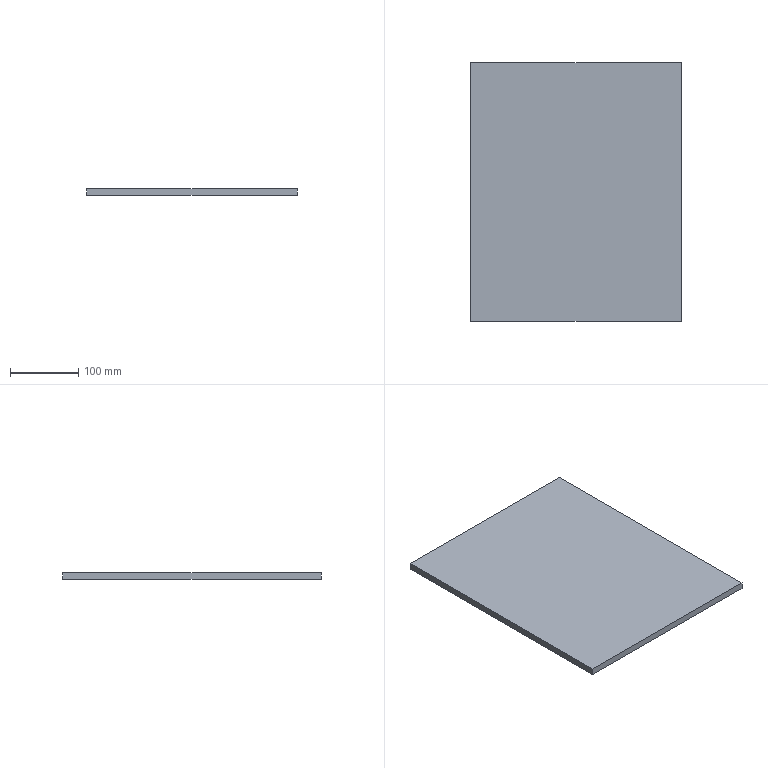Part | STEP file | 机台DoorPlate-单元二 | 1 solid | 6 faces | box 310 x 380 x 10 mm | volume 1178000 mm3 | plane 6
STEP:
#1=CARTESIAN_POINT('',(0.,0.,0.));
#2=DIRECTION('',(0.,0.,1.));
#3=DIRECTION('',(1.,0.,0.));
#4=AXIS2_PLACEMENT_3D('',#1,#2,#3);
#5=CARTESIAN_POINT('',(155.,-190.,0.));
#6=VERTEX_POINT('',#5);
#7=CARTESIAN_POINT('',(155.,190.,0.));
#8=VERTEX_POINT('',#7);
#9=CARTESIAN_POINT('',(155.,-190.,0.));
#10=DIRECTION('',(0.,1.,0.));
#11=VECTOR('',#10,1.);
#12=LINE('',#9,#11);
#13=CARTESIAN_POINT('',(155.,-190.,10.));
#14=DIRECTION('',(-1.,0.,0.));
#15=DIRECTION('',(0.,0.,1.));
#16=AXIS2_PLACEMENT_3D('',#13,#14,#15);
#17=PLANE('',#16);
#18=CARTESIAN_POINT('',(-10.,0.));
#19=DIRECTION('',(0.,1.));
#20=VECTOR('',#19,1.);
#21=LINE('',#18,#20);
#22=(GEOMETRIC_REPRESENTATION_CONTEXT(2)PARAMETRIC_REPRESENTATION_CONTEXT()REPRESENTATION_CONTEXT('',''));
#23=DEFINITIONAL_REPRESENTATION('',(#21),#22);
#24=PCURVE('',#17,#23);
#25=CARTESIAN_POINT('',(0.,0.,0.));
#26=DIRECTION('',(0.,0.,-1.));
#27=DIRECTION('',(-1.,0.,0.));
#28=AXIS2_PLACEMENT_3D('',#25,#26,#27);
#29=PLANE('',#28);
#30=CARTESIAN_POINT('',(-155.,-190.));
#31=DIRECTION('',(0.,1.));
#32=VECTOR('',#31,1.);
#33=LINE('',#30,#32);
#34=(GEOMETRIC_REPRESENTATION_CONTEXT(2)PARAMETRIC_REPRESENTATION_CONTEXT()REPRESENTATION_CONTEXT('',''));
#35=DEFINITIONAL_REPRESENTATION('',(#33),#34);
#36=PCURVE('',#29,#35);
#37=SURFACE_CURVE('',#12,(#24,#36),.PCURVE_S1.);
#38=EDGE_CURVE('',#6,#8,#37,.T.);
#39=ORIENTED_EDGE('',*,*,#38,.T.);
#40=CARTESIAN_POINT('',(155.,190.,10.));
#41=VERTEX_POINT('',#40);
#42=CARTESIAN_POINT('',(155.,190.,10.));
#43=DIRECTION('',(0.,0.,-1.));
#44=VECTOR('',#43,1.);
#45=LINE('',#42,#44);
#46=CARTESIAN_POINT('',(0.,380.));
#47=DIRECTION('',(-1.,0.));
#48=VECTOR('',#47,1.);
#49=LINE('',#46,#48);
#50=(GEOMETRIC_REPRESENTATION_CONTEXT(2)PARAMETRIC_REPRESENTATION_CONTEXT()REPRESENTATION_CONTEXT('',''));
#51=DEFINITIONAL_REPRESENTATION('',(#49),#50);
#52=PCURVE('',#17,#51);
#53=CARTESIAN_POINT('',(-155.,190.,10.));
#54=DIRECTION('',(0.,-1.,0.));
#55=DIRECTION('',(0.,0.,-1.));
#56=AXIS2_PLACEMENT_3D('',#53,#54,#55);
#57=PLANE('',#56);
#58=CARTESIAN_POINT('',(0.,310.));
#59=DIRECTION('',(1.,0.));
#60=VECTOR('',#59,1.);
#61=LINE('',#58,#60);
#62=(GEOMETRIC_REPRESENTATION_CONTEXT(2)PARAMETRIC_REPRESENTATION_CONTEXT()REPRESENTATION_CONTEXT('',''));
#63=DEFINITIONAL_REPRESENTATION('',(#61),#62);
#64=PCURVE('',#57,#63);
#65=SURFACE_CURVE('',#45,(#52,#64),.PCURVE_S1.);
#66=EDGE_CURVE('',#41,#8,#65,.T.);
#67=ORIENTED_EDGE('',*,*,#66,.F.);
#68=CARTESIAN_POINT('',(155.,-190.,10.));
#69=VERTEX_POINT('',#68);
#70=CARTESIAN_POINT('',(155.,-190.,10.));
#71=DIRECTION('',(0.,1.,0.));
#72=VECTOR('',#71,1.);
#73=LINE('',#70,#72);
#74=CARTESIAN_POINT('',(0.,0.));
#75=DIRECTION('',(0.,1.));
#76=VECTOR('',#75,1.);
#77=LINE('',#74,#76);
#78=(GEOMETRIC_REPRESENTATION_CONTEXT(2)PARAMETRIC_REPRESENTATION_CONTEXT()REPRESENTATION_CONTEXT('',''));
#79=DEFINITIONAL_REPRESENTATION('',(#77),#78);
#80=PCURVE('',#17,#79);
#81=CARTESIAN_POINT('',(0.,0.,10.));
#82=DIRECTION('',(0.,0.,-1.));
#83=DIRECTION('',(-1.,0.,0.));
#84=AXIS2_PLACEMENT_3D('',#81,#82,#83);
#85=PLANE('',#84);
#86=CARTESIAN_POINT('',(-155.,-190.));
#87=DIRECTION('',(0.,1.));
#88=VECTOR('',#87,1.);
#89=LINE('',#86,#88);
#90=(GEOMETRIC_REPRESENTATION_CONTEXT(2)PARAMETRIC_REPRESENTATION_CONTEXT()REPRESENTATION_CONTEXT('',''));
#91=DEFINITIONAL_REPRESENTATION('',(#89),#90);
#92=PCURVE('',#85,#91);
#93=SURFACE_CURVE('',#73,(#80,#92),.PCURVE_S1.);
#94=EDGE_CURVE('',#69,#41,#93,.T.);
#95=ORIENTED_EDGE('',*,*,#94,.F.);
#96=CARTESIAN_POINT('',(155.,-190.,10.));
#97=DIRECTION('',(0.,0.,-1.));
#98=VECTOR('',#97,1.);
#99=LINE('',#96,#98);
#100=CARTESIAN_POINT('',(0.,0.));
#101=DIRECTION('',(-1.,0.));
#102=VECTOR('',#101,1.);
#103=LINE('',#100,#102);
#104=(GEOMETRIC_REPRESENTATION_CONTEXT(2)PARAMETRIC_REPRESENTATION_CONTEXT()REPRESENTATION_CONTEXT('',''));
#105=DEFINITIONAL_REPRESENTATION('',(#103),#104);
#106=PCURVE('',#17,#105);
#107=CARTESIAN_POINT('',(-155.,-190.,10.));
#108=DIRECTION('',(0.,1.,0.));
#109=DIRECTION('',(0.,0.,1.));
#110=AXIS2_PLACEMENT_3D('',#107,#108,#109);
#111=PLANE('',#110);
#112=CARTESIAN_POINT('',(0.,310.));
#113=DIRECTION('',(-1.,0.));
#114=VECTOR('',#113,1.);
#115=LINE('',#112,#114);
#116=(GEOMETRIC_REPRESENTATION_CONTEXT(2)PARAMETRIC_REPRESENTATION_CONTEXT()REPRESENTATION_CONTEXT('',''));
#117=DEFINITIONAL_REPRESENTATION('',(#115),#116);
#118=PCURVE('',#111,#117);
#119=SURFACE_CURVE('',#99,(#106,#118),.PCURVE_S1.);
#120=EDGE_CURVE('',#69,#6,#119,.T.);
#121=ORIENTED_EDGE('',*,*,#120,.T.);
#122=EDGE_LOOP('',(#39,#67,#95,#121));
#123=FACE_BOUND('',#122,.T.);
#124=ADVANCED_FACE('',(#123),#17,.F.);
#125=CARTESIAN_POINT('',(-155.,190.,0.));
#126=VERTEX_POINT('',#125);
#127=CARTESIAN_POINT('',(-155.,190.,0.));
#128=DIRECTION('',(-1.,0.,0.));
#129=VECTOR('',#128,1.);
#130=LINE('',#127,#129);
#131=CARTESIAN_POINT('',(10.,0.));
#132=DIRECTION('',(0.,-1.));
#133=VECTOR('',#132,1.);
#134=LINE('',#131,#133);
#135=(GEOMETRIC_REPRESENTATION_CONTEXT(2)PARAMETRIC_REPRESENTATION_CONTEXT()REPRESENTATION_CONTEXT('',''));
#136=DEFINITIONAL_REPRESENTATION('',(#134),#135);
#137=PCURVE('',#57,#136);
#138=CARTESIAN_POINT('',(155.,190.));
#139=DIRECTION('',(1.,0.));
#140=VECTOR('',#139,1.);
#141=LINE('',#138,#140);
#142=(GEOMETRIC_REPRESENTATION_CONTEXT(2)PARAMETRIC_REPRESENTATION_CONTEXT()REPRESENTATION_CONTEXT('',''));
#143=DEFINITIONAL_REPRESENTATION('',(#141),#142);
#144=PCURVE('',#29,#143);
#145=SURFACE_CURVE('',#130,(#137,#144),.PCURVE_S1.);
#146=EDGE_CURVE('',#8,#126,#145,.T.);
#147=ORIENTED_EDGE('',*,*,#146,.T.);
#148=CARTESIAN_POINT('',(-155.,190.,10.));
#149=VERTEX_POINT('',#148);
#150=CARTESIAN_POINT('',(-155.,190.,10.));
#151=DIRECTION('',(0.,0.,-1.));
#152=VECTOR('',#151,1.);
#153=LINE('',#150,#152);
#154=CARTESIAN_POINT('',(0.,0.));
#155=DIRECTION('',(1.,0.));
#156=VECTOR('',#155,1.);
#157=LINE('',#154,#156);
#158=(GEOMETRIC_REPRESENTATION_CONTEXT(2)PARAMETRIC_REPRESENTATION_CONTEXT()REPRESENTATION_CONTEXT('',''));
#159=DEFINITIONAL_REPRESENTATION('',(#157),#158);
#160=PCURVE('',#57,#159);
#161=CARTESIAN_POINT('',(-155.,-190.,10.));
#162=DIRECTION('',(1.,0.,0.));
#163=DIRECTION('',(0.,0.,-1.));
#164=AXIS2_PLACEMENT_3D('',#161,#162,#163);
#165=PLANE('',#164);
#166=CARTESIAN_POINT('',(0.,380.));
#167=DIRECTION('',(1.,0.));
#168=VECTOR('',#167,1.);
#169=LINE('',#166,#168);
#170=(GEOMETRIC_REPRESENTATION_CONTEXT(2)PARAMETRIC_REPRESENTATION_CONTEXT()REPRESENTATION_CONTEXT('',''));
#171=DEFINITIONAL_REPRESENTATION('',(#169),#170);
#172=PCURVE('',#165,#171);
#173=SURFACE_CURVE('',#153,(#160,#172),.PCURVE_S1.);
#174=EDGE_CURVE('',#149,#126,#173,.T.);
#175=ORIENTED_EDGE('',*,*,#174,.F.);
#176=CARTESIAN_POINT('',(-155.,190.,10.));
#177=DIRECTION('',(-1.,0.,0.));
#178=VECTOR('',#177,1.);
#179=LINE('',#176,#178);
#180=CARTESIAN_POINT('',(0.,0.));
#181=DIRECTION('',(0.,-1.));
#182=VECTOR('',#181,1.);
#183=LINE('',#180,#182);
#184=(GEOMETRIC_REPRESENTATION_CONTEXT(2)PARAMETRIC_REPRESENTATION_CONTEXT()REPRESENTATION_CONTEXT('',''));
#185=DEFINITIONAL_REPRESENTATION('',(#183),#184);
#186=PCURVE('',#57,#185);
#187=CARTESIAN_POINT('',(155.,190.));
#188=DIRECTION('',(1.,0.));
#189=VECTOR('',#188,1.);
#190=LINE('',#187,#189);
#191=(GEOMETRIC_REPRESENTATION_CONTEXT(2)PARAMETRIC_REPRESENTATION_CONTEXT()REPRESENTATION_CONTEXT('',''));
#192=DEFINITIONAL_REPRESENTATION('',(#190),#191);
#193=PCURVE('',#85,#192);
#194=SURFACE_CURVE('',#179,(#186,#193),.PCURVE_S1.);
#195=EDGE_CURVE('',#41,#149,#194,.T.);
#196=ORIENTED_EDGE('',*,*,#195,.F.);
#197=ORIENTED_EDGE('',*,*,#66,.T.);
#198=EDGE_LOOP('',(#147,#175,#196,#197));
#199=FACE_BOUND('',#198,.T.);
#200=ADVANCED_FACE('',(#199),#57,.F.);
#201=CARTESIAN_POINT('',(-155.,-190.,0.));
#202=VERTEX_POINT('',#201);
#203=CARTESIAN_POINT('',(-155.,-190.,0.));
#204=DIRECTION('',(0.,-1.,0.));
#205=VECTOR('',#204,1.);
#206=LINE('',#203,#205);
#207=CARTESIAN_POINT('',(10.,0.));
#208=DIRECTION('',(0.,-1.));
#209=VECTOR('',#208,1.);
#210=LINE('',#207,#209);
#211=(GEOMETRIC_REPRESENTATION_CONTEXT(2)PARAMETRIC_REPRESENTATION_CONTEXT()REPRESENTATION_CONTEXT('',''));
#212=DEFINITIONAL_REPRESENTATION('',(#210),#211);
#213=PCURVE('',#165,#212);
#214=CARTESIAN_POINT('',(155.,-190.));
#215=DIRECTION('',(0.,-1.));
#216=VECTOR('',#215,1.);
#217=LINE('',#214,#216);
#218=(GEOMETRIC_REPRESENTATION_CONTEXT(2)PARAMETRIC_REPRESENTATION_CONTEXT()REPRESENTATION_CONTEXT('',''));
#219=DEFINITIONAL_REPRESENTATION('',(#217),#218);
#220=PCURVE('',#29,#219);
#221=SURFACE_CURVE('',#206,(#213,#220),.PCURVE_S1.);
#222=EDGE_CURVE('',#126,#202,#221,.T.);
#223=ORIENTED_EDGE('',*,*,#222,.T.);
#224=CARTESIAN_POINT('',(-155.,-190.,10.));
#225=VERTEX_POINT('',#224);
#226=CARTESIAN_POINT('',(-155.,-190.,10.));
#227=DIRECTION('',(0.,0.,-1.));
#228=VECTOR('',#227,1.);
#229=LINE('',#226,#228);
#230=CARTESIAN_POINT('',(0.,0.));
#231=DIRECTION('',(1.,0.));
#232=VECTOR('',#231,1.);
#233=LINE('',#230,#232);
#234=(GEOMETRIC_REPRESENTATION_CONTEXT(2)PARAMETRIC_REPRESENTATION_CONTEXT()REPRESENTATION_CONTEXT('',''));
#235=DEFINITIONAL_REPRESENTATION('',(#233),#234);
#236=PCURVE('',#165,#235);
#237=CARTESIAN_POINT('',(0.,0.));
#238=DIRECTION('',(-1.,0.));
#239=VECTOR('',#238,1.);
#240=LINE('',#237,#239);
#241=(GEOMETRIC_REPRESENTATION_CONTEXT(2)PARAMETRIC_REPRESENTATION_CONTEXT()REPRESENTATION_CONTEXT('',''));
#242=DEFINITIONAL_REPRESENTATION('',(#240),#241);
#243=PCURVE('',#111,#242);
#244=SURFACE_CURVE('',#229,(#236,#243),.PCURVE_S1.);
#245=EDGE_CURVE('',#225,#202,#244,.T.);
#246=ORIENTED_EDGE('',*,*,#245,.F.);
#247=CARTESIAN_POINT('',(-155.,-190.,10.));
#248=DIRECTION('',(0.,-1.,0.));
#249=VECTOR('',#248,1.);
#250=LINE('',#247,#249);
#251=CARTESIAN_POINT('',(0.,0.));
#252=DIRECTION('',(0.,-1.));
#253=VECTOR('',#252,1.);
#254=LINE('',#251,#253);
#255=(GEOMETRIC_REPRESENTATION_CONTEXT(2)PARAMETRIC_REPRESENTATION_CONTEXT()REPRESENTATION_CONTEXT('',''));
#256=DEFINITIONAL_REPRESENTATION('',(#254),#255);
#257=PCURVE('',#165,#256);
#258=CARTESIAN_POINT('',(155.,-190.));
#259=DIRECTION('',(0.,-1.));
#260=VECTOR('',#259,1.);
#261=LINE('',#258,#260);
#262=(GEOMETRIC_REPRESENTATION_CONTEXT(2)PARAMETRIC_REPRESENTATION_CONTEXT()REPRESENTATION_CONTEXT('',''));
#263=DEFINITIONAL_REPRESENTATION('',(#261),#262);
#264=PCURVE('',#85,#263);
#265=SURFACE_CURVE('',#250,(#257,#264),.PCURVE_S1.);
#266=EDGE_CURVE('',#149,#225,#265,.T.);
#267=ORIENTED_EDGE('',*,*,#266,.F.);
#268=ORIENTED_EDGE('',*,*,#174,.T.);
#269=EDGE_LOOP('',(#223,#246,#267,#268));
#270=FACE_BOUND('',#269,.T.);
#271=ADVANCED_FACE('',(#270),#165,.F.);
#272=CARTESIAN_POINT('',(-155.,-190.,0.));
#273=DIRECTION('',(1.,0.,0.));
#274=VECTOR('',#273,1.);
#275=LINE('',#272,#274);
#276=CARTESIAN_POINT('',(-10.,0.));
#277=DIRECTION('',(0.,1.));
#278=VECTOR('',#277,1.);
#279=LINE('',#276,#278);
#280=(GEOMETRIC_REPRESENTATION_CONTEXT(2)PARAMETRIC_REPRESENTATION_CONTEXT()REPRESENTATION_CONTEXT('',''));
#281=DEFINITIONAL_REPRESENTATION('',(#279),#280);
#282=PCURVE('',#111,#281);
#283=CARTESIAN_POINT('',(155.,-190.));
#284=DIRECTION('',(-1.,0.));
#285=VECTOR('',#284,1.);
#286=LINE('',#283,#285);
#287=(GEOMETRIC_REPRESENTATION_CONTEXT(2)PARAMETRIC_REPRESENTATION_CONTEXT()REPRESENTATION_CONTEXT('',''));
#288=DEFINITIONAL_REPRESENTATION('',(#286),#287);
#289=PCURVE('',#29,#288);
#290=SURFACE_CURVE('',#275,(#282,#289),.PCURVE_S1.);
#291=EDGE_CURVE('',#202,#6,#290,.T.);
#292=ORIENTED_EDGE('',*,*,#291,.T.);
#293=ORIENTED_EDGE('',*,*,#120,.F.);
#294=CARTESIAN_POINT('',(-155.,-190.,10.));
#295=DIRECTION('',(1.,0.,0.));
#296=VECTOR('',#295,1.);
#297=LINE('',#294,#296);
#298=CARTESIAN_POINT('',(0.,0.));
#299=DIRECTION('',(0.,1.));
#300=VECTOR('',#299,1.);
#301=LINE('',#298,#300);
#302=(GEOMETRIC_REPRESENTATION_CONTEXT(2)PARAMETRIC_REPRESENTATION_CONTEXT()REPRESENTATION_CONTEXT('',''));
#303=DEFINITIONAL_REPRESENTATION('',(#301),#302);
#304=PCURVE('',#111,#303);
#305=CARTESIAN_POINT('',(155.,-190.));
#306=DIRECTION('',(-1.,0.));
#307=VECTOR('',#306,1.);
#308=LINE('',#305,#307);
#309=(GEOMETRIC_REPRESENTATION_CONTEXT(2)PARAMETRIC_REPRESENTATION_CONTEXT()REPRESENTATION_CONTEXT('',''));
#310=DEFINITIONAL_REPRESENTATION('',(#308),#309);
#311=PCURVE('',#85,#310);
#312=SURFACE_CURVE('',#297,(#304,#311),.PCURVE_S1.);
#313=EDGE_CURVE('',#225,#69,#312,.T.);
#314=ORIENTED_EDGE('',*,*,#313,.F.);
#315=ORIENTED_EDGE('',*,*,#245,.T.);
#316=EDGE_LOOP('',(#292,#293,#314,#315));
#317=FACE_BOUND('',#316,.T.);
#318=ADVANCED_FACE('',(#317),#111,.F.);
#319=ORIENTED_EDGE('',*,*,#94,.T.);
#320=ORIENTED_EDGE('',*,*,#195,.T.);
#321=ORIENTED_EDGE('',*,*,#266,.T.);
#322=ORIENTED_EDGE('',*,*,#313,.T.);
#323=EDGE_LOOP('',(#319,#320,#321,#322));
#324=FACE_BOUND('',#323,.T.);
#325=ADVANCED_FACE('',(#324),#85,.F.);
#326=ORIENTED_EDGE('',*,*,#38,.F.);
#327=ORIENTED_EDGE('',*,*,#291,.F.);
#328=ORIENTED_EDGE('',*,*,#222,.F.);
#329=ORIENTED_EDGE('',*,*,#146,.F.);
#330=EDGE_LOOP('',(#326,#327,#328,#329));
#331=FACE_BOUND('',#330,.T.);
#332=ADVANCED_FACE('',(#331),#29,.T.);
#333=CLOSED_SHELL('',(#124,#200,#271,#318,#325,#332));
#334=MANIFOLD_SOLID_BREP('',#333);
#335=(LENGTH_UNIT()NAMED_UNIT(*)SI_UNIT(.MILLI.,.METRE.));
#336=UNCERTAINTY_MEASURE_WITH_UNIT(LENGTH_MEASURE(0.0000001),#335,'','');
#337=(NAMED_UNIT(*)PLANE_ANGLE_UNIT()SI_UNIT($,.RADIAN.));
#338=(NAMED_UNIT(*)SI_UNIT($,.STERADIAN.)SOLID_ANGLE_UNIT());
#339=(GEOMETRIC_REPRESENTATION_CONTEXT(3)GLOBAL_UNCERTAINTY_ASSIGNED_CONTEXT((#336))GLOBAL_UNIT_ASSIGNED_CONTEXT((#335,#337,#338))REPRESENTATION_CONTEXT('',''));
#340=ADVANCED_BREP_SHAPE_REPRESENTATION('',(#4,#334),#339);